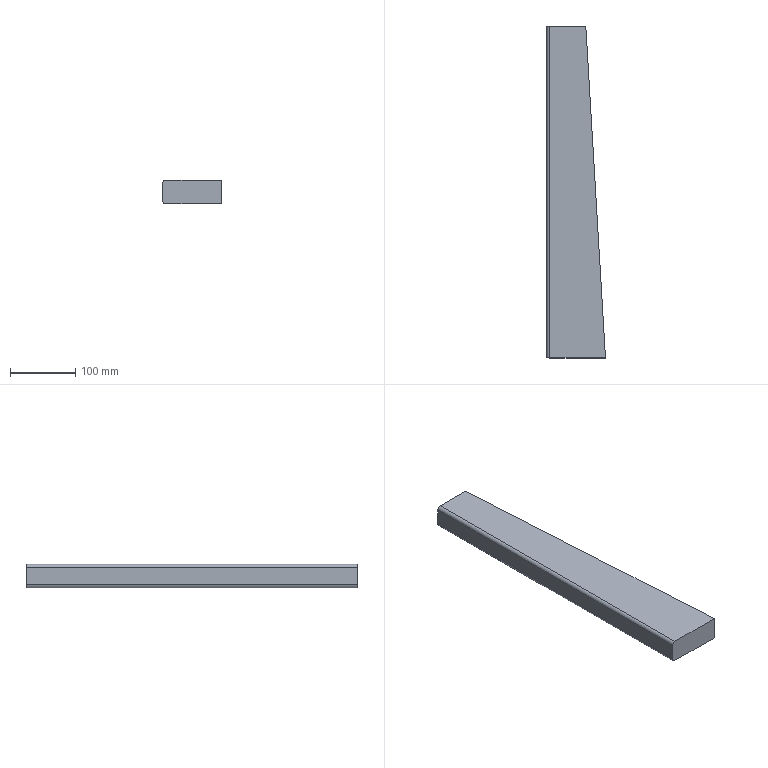Part | STEP file | 07-High-level comb rack 3 | 1 solid | 8 faces | box 90 x 507 x 36 mm | volume 1363460 mm3 | plane 6 | cylinder 2 | commonest cylinder face diameters 10 x2
STEP:
#1=CARTESIAN_POINT('',(0.,0.,0.));
#2=DIRECTION('',(0.,0.,1.));
#3=DIRECTION('',(1.,0.,0.));
#4=AXIS2_PLACEMENT_3D('',#1,#2,#3);
#5=CARTESIAN_POINT('',(0.,0.,31.));
#6=VERTEX_POINT('',#5);
#7=CARTESIAN_POINT('',(0.,0.,5.));
#8=VERTEX_POINT('',#7);
#9=CARTESIAN_POINT('',(0.,0.,36.));
#10=DIRECTION('',(0.,0.,-1.));
#11=VECTOR('',#10,1.);
#12=LINE('',#9,#11);
#13=CARTESIAN_POINT('',(0.,0.,36.));
#14=DIRECTION('',(1.,0.,0.));
#15=DIRECTION('',(0.,1.,0.));
#16=AXIS2_PLACEMENT_3D('',#13,#14,#15);
#17=PLANE('',#16);
#18=CARTESIAN_POINT('',(0.,0.));
#19=DIRECTION('',(0.,-1.));
#20=VECTOR('',#19,1.);
#21=LINE('',#18,#20);
#22=(GEOMETRIC_REPRESENTATION_CONTEXT(2)PARAMETRIC_REPRESENTATION_CONTEXT()REPRESENTATION_CONTEXT('',''));
#23=DEFINITIONAL_REPRESENTATION('',(#21),#22);
#24=PCURVE('',#17,#23);
#25=CARTESIAN_POINT('',(0.,0.,36.));
#26=DIRECTION('',(0.,-1.,0.));
#27=DIRECTION('',(0.,0.,-1.));
#28=AXIS2_PLACEMENT_3D('',#25,#26,#27);
#29=PLANE('',#28);
#30=CARTESIAN_POINT('',(0.,0.));
#31=DIRECTION('',(1.,0.));
#32=VECTOR('',#31,1.);
#33=LINE('',#30,#32);
#34=(GEOMETRIC_REPRESENTATION_CONTEXT(2)PARAMETRIC_REPRESENTATION_CONTEXT()REPRESENTATION_CONTEXT('',''));
#35=DEFINITIONAL_REPRESENTATION('',(#33),#34);
#36=PCURVE('',#29,#35);
#37=SURFACE_CURVE('',#12,(#24,#36),.PCURVE_S1.);
#38=EDGE_CURVE('',#6,#8,#37,.T.);
#39=ORIENTED_EDGE('',*,*,#38,.T.);
#40=CARTESIAN_POINT('',(0.,-507.,5.));
#41=VERTEX_POINT('',#40);
#42=CARTESIAN_POINT('',(0.,0.,5.));
#43=DIRECTION('',(0.,-1.,0.));
#44=VECTOR('',#43,1.);
#45=LINE('',#42,#44);
#46=CARTESIAN_POINT('',(0.,-31.));
#47=DIRECTION('',(-1.,0.));
#48=VECTOR('',#47,1.);
#49=LINE('',#46,#48);
#50=(GEOMETRIC_REPRESENTATION_CONTEXT(2)PARAMETRIC_REPRESENTATION_CONTEXT()REPRESENTATION_CONTEXT('',''));
#51=DEFINITIONAL_REPRESENTATION('',(#49),#50);
#52=PCURVE('',#17,#51);
#53=CARTESIAN_POINT('',(5.,0.,5.));
#54=DIRECTION('',(0.,-1.,0.));
#55=DIRECTION('',(1.,0.,0.));
#56=AXIS2_PLACEMENT_3D('',#53,#54,#55);
#57=CYLINDRICAL_SURFACE('',#56,5.);
#58=CARTESIAN_POINT('',(3.142,0.));
#59=DIRECTION('',(0.,1.));
#60=VECTOR('',#59,1.);
#61=LINE('',#58,#60);
#62=(GEOMETRIC_REPRESENTATION_CONTEXT(2)PARAMETRIC_REPRESENTATION_CONTEXT()REPRESENTATION_CONTEXT('',''));
#63=DEFINITIONAL_REPRESENTATION('',(#61),#62);
#64=PCURVE('',#57,#63);
#65=SURFACE_CURVE('',#45,(#52,#64),.PCURVE_S1.);
#66=EDGE_CURVE('',#8,#41,#65,.T.);
#67=ORIENTED_EDGE('',*,*,#66,.T.);
#68=CARTESIAN_POINT('',(0.,-507.,31.));
#69=VERTEX_POINT('',#68);
#70=CARTESIAN_POINT('',(0.,-507.,36.));
#71=DIRECTION('',(0.,0.,-1.));
#72=VECTOR('',#71,1.);
#73=LINE('',#70,#72);
#74=CARTESIAN_POINT('',(-507.,0.));
#75=DIRECTION('',(0.,-1.));
#76=VECTOR('',#75,1.);
#77=LINE('',#74,#76);
#78=(GEOMETRIC_REPRESENTATION_CONTEXT(2)PARAMETRIC_REPRESENTATION_CONTEXT()REPRESENTATION_CONTEXT('',''));
#79=DEFINITIONAL_REPRESENTATION('',(#77),#78);
#80=PCURVE('',#17,#79);
#81=CARTESIAN_POINT('',(0.,-507.,36.));
#82=DIRECTION('',(0.,1.,0.));
#83=DIRECTION('',(0.,0.,1.));
#84=AXIS2_PLACEMENT_3D('',#81,#82,#83);
#85=PLANE('',#84);
#86=CARTESIAN_POINT('',(0.,0.));
#87=DIRECTION('',(-1.,0.));
#88=VECTOR('',#87,1.);
#89=LINE('',#86,#88);
#90=(GEOMETRIC_REPRESENTATION_CONTEXT(2)PARAMETRIC_REPRESENTATION_CONTEXT()REPRESENTATION_CONTEXT('',''));
#91=DEFINITIONAL_REPRESENTATION('',(#89),#90);
#92=PCURVE('',#85,#91);
#93=SURFACE_CURVE('',#73,(#80,#92),.PCURVE_S1.);
#94=EDGE_CURVE('',#69,#41,#93,.T.);
#95=ORIENTED_EDGE('',*,*,#94,.F.);
#96=CARTESIAN_POINT('',(0.,0.,31.));
#97=DIRECTION('',(0.,1.,0.));
#98=VECTOR('',#97,1.);
#99=LINE('',#96,#98);
#100=CARTESIAN_POINT('',(0.,-5.));
#101=DIRECTION('',(1.,0.));
#102=VECTOR('',#101,1.);
#103=LINE('',#100,#102);
#104=(GEOMETRIC_REPRESENTATION_CONTEXT(2)PARAMETRIC_REPRESENTATION_CONTEXT()REPRESENTATION_CONTEXT('',''));
#105=DEFINITIONAL_REPRESENTATION('',(#103),#104);
#106=PCURVE('',#17,#105);
#107=CARTESIAN_POINT('',(5.,0.,31.));
#108=DIRECTION('',(0.,1.,0.));
#109=DIRECTION('',(-1.,0.,0.));
#110=AXIS2_PLACEMENT_3D('',#107,#108,#109);
#111=CYLINDRICAL_SURFACE('',#110,5.);
#112=CARTESIAN_POINT('',(0.,0.));
#113=DIRECTION('',(0.,1.));
#114=VECTOR('',#113,1.);
#115=LINE('',#112,#114);
#116=(GEOMETRIC_REPRESENTATION_CONTEXT(2)PARAMETRIC_REPRESENTATION_CONTEXT()REPRESENTATION_CONTEXT('',''));
#117=DEFINITIONAL_REPRESENTATION('',(#115),#116);
#118=PCURVE('',#111,#117);
#119=SURFACE_CURVE('',#99,(#106,#118),.PCURVE_S1.);
#120=EDGE_CURVE('',#69,#6,#119,.T.);
#121=ORIENTED_EDGE('',*,*,#120,.T.);
#122=EDGE_LOOP('',(#39,#67,#95,#121));
#123=FACE_BOUND('',#122,.T.);
#124=ADVANCED_FACE('',(#123),#17,.F.);
#125=ORIENTED_EDGE('',*,*,#94,.T.);
#126=CARTESIAN_POINT('',(5.,-507.,0.));
#127=VERTEX_POINT('',#126);
#128=CARTESIAN_POINT('',(5.,-507.,5.));
#129=DIRECTION('',(0.,-1.,0.));
#130=DIRECTION('',(0.,0.,1.));
#131=AXIS2_PLACEMENT_3D('',#128,#129,#130);
#132=CIRCLE('',#131,5.);
#133=CARTESIAN_POINT('',(-26.,5.));
#134=CARTESIAN_POINT('',(-26.,-3.66));
#135=CARTESIAN_POINT('',(-33.5,0.6699));
#136=CARTESIAN_POINT('',(-41.,5.));
#137=CARTESIAN_POINT('',(-33.5,9.33));
#138=CARTESIAN_POINT('',(-26.,13.66));
#139=CARTESIAN_POINT('',(-26.,5.));
#140=(BOUNDED_CURVE()B_SPLINE_CURVE(2,(#133,#134,#135,#136,#137,#138,#139),.UNSPECIFIED.,.T.,.F.)B_SPLINE_CURVE_WITH_KNOTS((1,2,2,2,2,1),(-2.094,0.,2.094,4.189,6.283,8.378),.UNSPECIFIED.)CURVE()GEOMETRIC_REPRESENTATION_ITEM()RATIONAL_B_SPLINE_CURVE((1.,0.5,1.,0.5,1.,0.5,1.))REPRESENTATION_ITEM(''));
#141=(GEOMETRIC_REPRESENTATION_CONTEXT(2)PARAMETRIC_REPRESENTATION_CONTEXT()REPRESENTATION_CONTEXT('',''));
#142=DEFINITIONAL_REPRESENTATION('',(#140),#141);
#143=PCURVE('',#85,#142);
#144=CARTESIAN_POINT('',(1.571,507.));
#145=DIRECTION('',(1.,0.));
#146=VECTOR('',#145,1.);
#147=LINE('',#144,#146);
#148=(GEOMETRIC_REPRESENTATION_CONTEXT(2)PARAMETRIC_REPRESENTATION_CONTEXT()REPRESENTATION_CONTEXT('',''));
#149=DEFINITIONAL_REPRESENTATION('',(#147),#148);
#150=PCURVE('',#57,#149);
#151=SURFACE_CURVE('',#132,(#143,#150),.PCURVE_S1.);
#152=EDGE_CURVE('',#41,#127,#151,.T.);
#153=ORIENTED_EDGE('',*,*,#152,.T.);
#154=CARTESIAN_POINT('',(90.,-507.,0.));
#155=VERTEX_POINT('',#154);
#156=CARTESIAN_POINT('',(0.,-507.,0.));
#157=DIRECTION('',(1.,0.,0.));
#158=VECTOR('',#157,1.);
#159=LINE('',#156,#158);
#160=CARTESIAN_POINT('',(-36.,0.));
#161=DIRECTION('',(0.,1.));
#162=VECTOR('',#161,1.);
#163=LINE('',#160,#162);
#164=(GEOMETRIC_REPRESENTATION_CONTEXT(2)PARAMETRIC_REPRESENTATION_CONTEXT()REPRESENTATION_CONTEXT('',''));
#165=DEFINITIONAL_REPRESENTATION('',(#163),#164);
#166=PCURVE('',#85,#165);
#167=CARTESIAN_POINT('',(0.,0.,0.));
#168=DIRECTION('',(0.,0.,1.));
#169=DIRECTION('',(1.,0.,0.));
#170=AXIS2_PLACEMENT_3D('',#167,#168,#169);
#171=PLANE('',#170);
#172=CARTESIAN_POINT('',(0.,-507.));
#173=DIRECTION('',(1.,0.));
#174=VECTOR('',#173,1.);
#175=LINE('',#172,#174);
#176=(GEOMETRIC_REPRESENTATION_CONTEXT(2)PARAMETRIC_REPRESENTATION_CONTEXT()REPRESENTATION_CONTEXT('',''));
#177=DEFINITIONAL_REPRESENTATION('',(#175),#176);
#178=PCURVE('',#171,#177);
#179=SURFACE_CURVE('',#159,(#166,#178),.PCURVE_S1.);
#180=EDGE_CURVE('',#127,#155,#179,.T.);
#181=ORIENTED_EDGE('',*,*,#180,.T.);
#182=CARTESIAN_POINT('',(90.,-507.,36.));
#183=VERTEX_POINT('',#182);
#184=CARTESIAN_POINT('',(90.,-507.,36.));
#185=DIRECTION('',(0.,0.,-1.));
#186=VECTOR('',#185,1.);
#187=LINE('',#184,#186);
#188=CARTESIAN_POINT('',(0.,90.));
#189=DIRECTION('',(-1.,0.));
#190=VECTOR('',#189,1.);
#191=LINE('',#188,#190);
#192=(GEOMETRIC_REPRESENTATION_CONTEXT(2)PARAMETRIC_REPRESENTATION_CONTEXT()REPRESENTATION_CONTEXT('',''));
#193=DEFINITIONAL_REPRESENTATION('',(#191),#192);
#194=PCURVE('',#85,#193);
#195=CARTESIAN_POINT('',(60.,0.,36.));
#196=DIRECTION('',(-0.9983,-0.05907,0.));
#197=DIRECTION('',(0.05907,-0.9983,0.));
#198=AXIS2_PLACEMENT_3D('',#195,#196,#197);
#199=PLANE('',#198);
#200=CARTESIAN_POINT('',(507.887,0.));
#201=DIRECTION('',(0.,-1.));
#202=VECTOR('',#201,1.);
#203=LINE('',#200,#202);
#204=(GEOMETRIC_REPRESENTATION_CONTEXT(2)PARAMETRIC_REPRESENTATION_CONTEXT()REPRESENTATION_CONTEXT('',''));
#205=DEFINITIONAL_REPRESENTATION('',(#203),#204);
#206=PCURVE('',#199,#205);
#207=SURFACE_CURVE('',#187,(#194,#206),.PCURVE_S1.);
#208=EDGE_CURVE('',#183,#155,#207,.T.);
#209=ORIENTED_EDGE('',*,*,#208,.F.);
#210=CARTESIAN_POINT('',(5.,-507.,36.));
#211=VERTEX_POINT('',#210);
#212=CARTESIAN_POINT('',(0.,-507.,36.));
#213=DIRECTION('',(1.,0.,0.));
#214=VECTOR('',#213,1.);
#215=LINE('',#212,#214);
#216=CARTESIAN_POINT('',(0.,0.));
#217=DIRECTION('',(0.,1.));
#218=VECTOR('',#217,1.);
#219=LINE('',#216,#218);
#220=(GEOMETRIC_REPRESENTATION_CONTEXT(2)PARAMETRIC_REPRESENTATION_CONTEXT()REPRESENTATION_CONTEXT('',''));
#221=DEFINITIONAL_REPRESENTATION('',(#219),#220);
#222=PCURVE('',#85,#221);
#223=CARTESIAN_POINT('',(0.,0.,36.));
#224=DIRECTION('',(0.,0.,1.));
#225=DIRECTION('',(1.,0.,0.));
#226=AXIS2_PLACEMENT_3D('',#223,#224,#225);
#227=PLANE('',#226);
#228=CARTESIAN_POINT('',(0.,-507.));
#229=DIRECTION('',(1.,0.));
#230=VECTOR('',#229,1.);
#231=LINE('',#228,#230);
#232=(GEOMETRIC_REPRESENTATION_CONTEXT(2)PARAMETRIC_REPRESENTATION_CONTEXT()REPRESENTATION_CONTEXT('',''));
#233=DEFINITIONAL_REPRESENTATION('',(#231),#232);
#234=PCURVE('',#227,#233);
#235=SURFACE_CURVE('',#215,(#222,#234),.PCURVE_S1.);
#236=EDGE_CURVE('',#211,#183,#235,.T.);
#237=ORIENTED_EDGE('',*,*,#236,.F.);
#238=CARTESIAN_POINT('',(5.,-507.,31.));
#239=DIRECTION('',(0.,-1.,0.));
#240=DIRECTION('',(0.,0.,1.));
#241=AXIS2_PLACEMENT_3D('',#238,#239,#240);
#242=CIRCLE('',#241,5.);
#243=CARTESIAN_POINT('',(0.,5.));
#244=CARTESIAN_POINT('',(0.,-3.66));
#245=CARTESIAN_POINT('',(-7.5,0.6699));
#246=CARTESIAN_POINT('',(-15.,5.));
#247=CARTESIAN_POINT('',(-7.5,9.33));
#248=CARTESIAN_POINT('',(0.,13.66));
#249=CARTESIAN_POINT('',(0.,5.));
#250=(BOUNDED_CURVE()B_SPLINE_CURVE(2,(#243,#244,#245,#246,#247,#248,#249),.UNSPECIFIED.,.T.,.F.)B_SPLINE_CURVE_WITH_KNOTS((1,2,2,2,2,1),(-2.094,0.,2.094,4.189,6.283,8.378),.UNSPECIFIED.)CURVE()GEOMETRIC_REPRESENTATION_ITEM()RATIONAL_B_SPLINE_CURVE((1.,0.5,1.,0.5,1.,0.5,1.))REPRESENTATION_ITEM(''));
#251=(GEOMETRIC_REPRESENTATION_CONTEXT(2)PARAMETRIC_REPRESENTATION_CONTEXT()REPRESENTATION_CONTEXT('',''));
#252=DEFINITIONAL_REPRESENTATION('',(#250),#251);
#253=PCURVE('',#85,#252);
#254=CARTESIAN_POINT('',(1.571,-507.));
#255=DIRECTION('',(-1.,0.));
#256=VECTOR('',#255,1.);
#257=LINE('',#254,#256);
#258=(GEOMETRIC_REPRESENTATION_CONTEXT(2)PARAMETRIC_REPRESENTATION_CONTEXT()REPRESENTATION_CONTEXT('',''));
#259=DEFINITIONAL_REPRESENTATION('',(#257),#258);
#260=PCURVE('',#111,#259);
#261=SURFACE_CURVE('',#242,(#253,#260),.PCURVE_S1.);
#262=EDGE_CURVE('',#211,#69,#261,.T.);
#263=ORIENTED_EDGE('',*,*,#262,.T.);
#264=EDGE_LOOP('',(#125,#153,#181,#209,#237,#263));
#265=FACE_BOUND('',#264,.T.);
#266=ADVANCED_FACE('',(#265),#85,.F.);
#267=CARTESIAN_POINT('',(60.,0.,0.));
#268=VERTEX_POINT('',#267);
#269=CARTESIAN_POINT('',(60.,0.,0.));
#270=DIRECTION('',(-0.05907,0.9983,0.));
#271=VECTOR('',#270,1.);
#272=LINE('',#269,#271);
#273=CARTESIAN_POINT('',(0.,-36.));
#274=DIRECTION('',(-1.,0.));
#275=VECTOR('',#274,1.);
#276=LINE('',#273,#275);
#277=(GEOMETRIC_REPRESENTATION_CONTEXT(2)PARAMETRIC_REPRESENTATION_CONTEXT()REPRESENTATION_CONTEXT('',''));
#278=DEFINITIONAL_REPRESENTATION('',(#276),#277);
#279=PCURVE('',#199,#278);
#280=CARTESIAN_POINT('',(60.,0.));
#281=DIRECTION('',(-0.05907,0.9983));
#282=VECTOR('',#281,1.);
#283=LINE('',#280,#282);
#284=(GEOMETRIC_REPRESENTATION_CONTEXT(2)PARAMETRIC_REPRESENTATION_CONTEXT()REPRESENTATION_CONTEXT('',''));
#285=DEFINITIONAL_REPRESENTATION('',(#283),#284);
#286=PCURVE('',#171,#285);
#287=SURFACE_CURVE('',#272,(#279,#286),.PCURVE_S1.);
#288=EDGE_CURVE('',#155,#268,#287,.T.);
#289=ORIENTED_EDGE('',*,*,#288,.T.);
#290=CARTESIAN_POINT('',(60.,0.,36.));
#291=VERTEX_POINT('',#290);
#292=CARTESIAN_POINT('',(60.,0.,36.));
#293=DIRECTION('',(0.,0.,-1.));
#294=VECTOR('',#293,1.);
#295=LINE('',#292,#294);
#296=CARTESIAN_POINT('',(0.,0.));
#297=DIRECTION('',(0.,-1.));
#298=VECTOR('',#297,1.);
#299=LINE('',#296,#298);
#300=(GEOMETRIC_REPRESENTATION_CONTEXT(2)PARAMETRIC_REPRESENTATION_CONTEXT()REPRESENTATION_CONTEXT('',''));
#301=DEFINITIONAL_REPRESENTATION('',(#299),#300);
#302=PCURVE('',#199,#301);
#303=CARTESIAN_POINT('',(0.,60.));
#304=DIRECTION('',(1.,0.));
#305=VECTOR('',#304,1.);
#306=LINE('',#303,#305);
#307=(GEOMETRIC_REPRESENTATION_CONTEXT(2)PARAMETRIC_REPRESENTATION_CONTEXT()REPRESENTATION_CONTEXT('',''));
#308=DEFINITIONAL_REPRESENTATION('',(#306),#307);
#309=PCURVE('',#29,#308);
#310=SURFACE_CURVE('',#295,(#302,#309),.PCURVE_S1.);
#311=EDGE_CURVE('',#291,#268,#310,.T.);
#312=ORIENTED_EDGE('',*,*,#311,.F.);
#313=CARTESIAN_POINT('',(60.,0.,36.));
#314=DIRECTION('',(-0.05907,0.9983,0.));
#315=VECTOR('',#314,1.);
#316=LINE('',#313,#315);
#317=CARTESIAN_POINT('',(0.,0.));
#318=DIRECTION('',(-1.,0.));
#319=VECTOR('',#318,1.);
#320=LINE('',#317,#319);
#321=(GEOMETRIC_REPRESENTATION_CONTEXT(2)PARAMETRIC_REPRESENTATION_CONTEXT()REPRESENTATION_CONTEXT('',''));
#322=DEFINITIONAL_REPRESENTATION('',(#320),#321);
#323=PCURVE('',#199,#322);
#324=CARTESIAN_POINT('',(60.,0.));
#325=DIRECTION('',(-0.05907,0.9983));
#326=VECTOR('',#325,1.);
#327=LINE('',#324,#326);
#328=(GEOMETRIC_REPRESENTATION_CONTEXT(2)PARAMETRIC_REPRESENTATION_CONTEXT()REPRESENTATION_CONTEXT('',''));
#329=DEFINITIONAL_REPRESENTATION('',(#327),#328);
#330=PCURVE('',#227,#329);
#331=SURFACE_CURVE('',#316,(#323,#330),.PCURVE_S1.);
#332=EDGE_CURVE('',#183,#291,#331,.T.);
#333=ORIENTED_EDGE('',*,*,#332,.F.);
#334=ORIENTED_EDGE('',*,*,#208,.T.);
#335=EDGE_LOOP('',(#289,#312,#333,#334));
#336=FACE_BOUND('',#335,.T.);
#337=ADVANCED_FACE('',(#336),#199,.F.);
#338=CARTESIAN_POINT('',(5.,0.,0.));
#339=VERTEX_POINT('',#338);
#340=CARTESIAN_POINT('',(0.,0.,0.));
#341=DIRECTION('',(-1.,0.,0.));
#342=VECTOR('',#341,1.);
#343=LINE('',#340,#342);
#344=CARTESIAN_POINT('',(36.,0.));
#345=DIRECTION('',(0.,-1.));
#346=VECTOR('',#345,1.);
#347=LINE('',#344,#346);
#348=(GEOMETRIC_REPRESENTATION_CONTEXT(2)PARAMETRIC_REPRESENTATION_CONTEXT()REPRESENTATION_CONTEXT('',''));
#349=DEFINITIONAL_REPRESENTATION('',(#347),#348);
#350=PCURVE('',#29,#349);
#351=CARTESIAN_POINT('',(0.,0.));
#352=DIRECTION('',(-1.,0.));
#353=VECTOR('',#352,1.);
#354=LINE('',#351,#353);
#355=(GEOMETRIC_REPRESENTATION_CONTEXT(2)PARAMETRIC_REPRESENTATION_CONTEXT()REPRESENTATION_CONTEXT('',''));
#356=DEFINITIONAL_REPRESENTATION('',(#354),#355);
#357=PCURVE('',#171,#356);
#358=SURFACE_CURVE('',#343,(#350,#357),.PCURVE_S1.);
#359=EDGE_CURVE('',#268,#339,#358,.T.);
#360=ORIENTED_EDGE('',*,*,#359,.T.);
#361=CARTESIAN_POINT('',(5.,0.,5.));
#362=DIRECTION('',(0.,1.,0.));
#363=DIRECTION('',(0.,0.,-1.));
#364=AXIS2_PLACEMENT_3D('',#361,#362,#363);
#365=CIRCLE('',#364,5.);
#366=CARTESIAN_POINT('',(36.,5.));
#367=CARTESIAN_POINT('',(36.,-3.66));
#368=CARTESIAN_POINT('',(28.5,0.6699));
#369=CARTESIAN_POINT('',(21.,5.));
#370=CARTESIAN_POINT('',(28.5,9.33));
#371=CARTESIAN_POINT('',(36.,13.66));
#372=CARTESIAN_POINT('',(36.,5.));
#373=(BOUNDED_CURVE()B_SPLINE_CURVE(2,(#366,#367,#368,#369,#370,#371,#372),.UNSPECIFIED.,.T.,.F.)B_SPLINE_CURVE_WITH_KNOTS((1,2,2,2,2,1),(-2.094,0.,2.094,4.189,6.283,8.378),.UNSPECIFIED.)CURVE()GEOMETRIC_REPRESENTATION_ITEM()RATIONAL_B_SPLINE_CURVE((1.,0.5,1.,0.5,1.,0.5,1.))REPRESENTATION_ITEM(''));
#374=(GEOMETRIC_REPRESENTATION_CONTEXT(2)PARAMETRIC_REPRESENTATION_CONTEXT()REPRESENTATION_CONTEXT('',''));
#375=DEFINITIONAL_REPRESENTATION('',(#373),#374);
#376=PCURVE('',#29,#375);
#377=CARTESIAN_POINT('',(4.712,0.));
#378=DIRECTION('',(-1.,0.));
#379=VECTOR('',#378,1.);
#380=LINE('',#377,#379);
#381=(GEOMETRIC_REPRESENTATION_CONTEXT(2)PARAMETRIC_REPRESENTATION_CONTEXT()REPRESENTATION_CONTEXT('',''));
#382=DEFINITIONAL_REPRESENTATION('',(#380),#381);
#383=PCURVE('',#57,#382);
#384=SURFACE_CURVE('',#365,(#376,#383),.PCURVE_S1.);
#385=EDGE_CURVE('',#339,#8,#384,.T.);
#386=ORIENTED_EDGE('',*,*,#385,.T.);
#387=ORIENTED_EDGE('',*,*,#38,.F.);
#388=CARTESIAN_POINT('',(5.,0.,36.));
#389=VERTEX_POINT('',#388);
#390=CARTESIAN_POINT('',(5.,0.,31.));
#391=DIRECTION('',(0.,1.,0.));
#392=DIRECTION('',(0.,0.,-1.));
#393=AXIS2_PLACEMENT_3D('',#390,#391,#392);
#394=CIRCLE('',#393,5.);
#395=CARTESIAN_POINT('',(10.,5.));
#396=CARTESIAN_POINT('',(10.,-3.66));
#397=CARTESIAN_POINT('',(2.5,0.6699));
#398=CARTESIAN_POINT('',(-5.,5.));
#399=CARTESIAN_POINT('',(2.5,9.33));
#400=CARTESIAN_POINT('',(10.,13.66));
#401=CARTESIAN_POINT('',(10.,5.));
#402=(BOUNDED_CURVE()B_SPLINE_CURVE(2,(#395,#396,#397,#398,#399,#400,#401),.UNSPECIFIED.,.T.,.F.)B_SPLINE_CURVE_WITH_KNOTS((1,2,2,2,2,1),(-2.094,0.,2.094,4.189,6.283,8.378),.UNSPECIFIED.)CURVE()GEOMETRIC_REPRESENTATION_ITEM()RATIONAL_B_SPLINE_CURVE((1.,0.5,1.,0.5,1.,0.5,1.))REPRESENTATION_ITEM(''));
#403=(GEOMETRIC_REPRESENTATION_CONTEXT(2)PARAMETRIC_REPRESENTATION_CONTEXT()REPRESENTATION_CONTEXT('',''));
#404=DEFINITIONAL_REPRESENTATION('',(#402),#403);
#405=PCURVE('',#29,#404);
#406=CARTESIAN_POINT('',(-1.571,0.));
#407=DIRECTION('',(1.,0.));
#408=VECTOR('',#407,1.);
#409=LINE('',#406,#408);
#410=(GEOMETRIC_REPRESENTATION_CONTEXT(2)PARAMETRIC_REPRESENTATION_CONTEXT()REPRESENTATION_CONTEXT('',''));
#411=DEFINITIONAL_REPRESENTATION('',(#409),#410);
#412=PCURVE('',#111,#411);
#413=SURFACE_CURVE('',#394,(#405,#412),.PCURVE_S1.);
#414=EDGE_CURVE('',#6,#389,#413,.T.);
#415=ORIENTED_EDGE('',*,*,#414,.T.);
#416=CARTESIAN_POINT('',(0.,0.,36.));
#417=DIRECTION('',(-1.,0.,0.));
#418=VECTOR('',#417,1.);
#419=LINE('',#416,#418);
#420=CARTESIAN_POINT('',(0.,0.));
#421=DIRECTION('',(0.,-1.));
#422=VECTOR('',#421,1.);
#423=LINE('',#420,#422);
#424=(GEOMETRIC_REPRESENTATION_CONTEXT(2)PARAMETRIC_REPRESENTATION_CONTEXT()REPRESENTATION_CONTEXT('',''));
#425=DEFINITIONAL_REPRESENTATION('',(#423),#424);
#426=PCURVE('',#29,#425);
#427=CARTESIAN_POINT('',(0.,0.));
#428=DIRECTION('',(-1.,0.));
#429=VECTOR('',#428,1.);
#430=LINE('',#427,#429);
#431=(GEOMETRIC_REPRESENTATION_CONTEXT(2)PARAMETRIC_REPRESENTATION_CONTEXT()REPRESENTATION_CONTEXT('',''));
#432=DEFINITIONAL_REPRESENTATION('',(#430),#431);
#433=PCURVE('',#227,#432);
#434=SURFACE_CURVE('',#419,(#426,#433),.PCURVE_S1.);
#435=EDGE_CURVE('',#291,#389,#434,.T.);
#436=ORIENTED_EDGE('',*,*,#435,.F.);
#437=ORIENTED_EDGE('',*,*,#311,.T.);
#438=EDGE_LOOP('',(#360,#386,#387,#415,#436,#437));
#439=FACE_BOUND('',#438,.T.);
#440=ADVANCED_FACE('',(#439),#29,.F.);
#441=ORIENTED_EDGE('',*,*,#435,.T.);
#442=CARTESIAN_POINT('',(5.,-507.,36.));
#443=DIRECTION('',(0.,-1.,0.));
#444=VECTOR('',#443,1.);
#445=LINE('',#442,#444);
#446=CARTESIAN_POINT('',(5.,-507.));
#447=DIRECTION('',(0.,-1.));
#448=VECTOR('',#447,1.);
#449=LINE('',#446,#448);
#450=(GEOMETRIC_REPRESENTATION_CONTEXT(2)PARAMETRIC_REPRESENTATION_CONTEXT()REPRESENTATION_CONTEXT('',''));
#451=DEFINITIONAL_REPRESENTATION('',(#449),#450);
#452=PCURVE('',#227,#451);
#453=CARTESIAN_POINT('',(1.571,-507.));
#454=DIRECTION('',(0.,-1.));
#455=VECTOR('',#454,1.);
#456=LINE('',#453,#455);
#457=(GEOMETRIC_REPRESENTATION_CONTEXT(2)PARAMETRIC_REPRESENTATION_CONTEXT()REPRESENTATION_CONTEXT('',''));
#458=DEFINITIONAL_REPRESENTATION('',(#456),#457);
#459=PCURVE('',#111,#458);
#460=SURFACE_CURVE('',#445,(#452,#459),.PCURVE_S1.);
#461=EDGE_CURVE('',#389,#211,#460,.T.);
#462=ORIENTED_EDGE('',*,*,#461,.T.);
#463=ORIENTED_EDGE('',*,*,#236,.T.);
#464=ORIENTED_EDGE('',*,*,#332,.T.);
#465=EDGE_LOOP('',(#441,#462,#463,#464));
#466=FACE_BOUND('',#465,.T.);
#467=ADVANCED_FACE('',(#466),#227,.T.);
#468=ORIENTED_EDGE('',*,*,#180,.F.);
#469=CARTESIAN_POINT('',(5.,0.,0.));
#470=DIRECTION('',(0.,1.,0.));
#471=VECTOR('',#470,1.);
#472=LINE('',#469,#471);
#473=CARTESIAN_POINT('',(5.,0.));
#474=DIRECTION('',(0.,1.));
#475=VECTOR('',#474,1.);
#476=LINE('',#473,#475);
#477=(GEOMETRIC_REPRESENTATION_CONTEXT(2)PARAMETRIC_REPRESENTATION_CONTEXT()REPRESENTATION_CONTEXT('',''));
#478=DEFINITIONAL_REPRESENTATION('',(#476),#477);
#479=PCURVE('',#171,#478);
#480=CARTESIAN_POINT('',(4.712,0.));
#481=DIRECTION('',(0.,-1.));
#482=VECTOR('',#481,1.);
#483=LINE('',#480,#482);
#484=(GEOMETRIC_REPRESENTATION_CONTEXT(2)PARAMETRIC_REPRESENTATION_CONTEXT()REPRESENTATION_CONTEXT('',''));
#485=DEFINITIONAL_REPRESENTATION('',(#483),#484);
#486=PCURVE('',#57,#485);
#487=SURFACE_CURVE('',#472,(#479,#486),.PCURVE_S1.);
#488=EDGE_CURVE('',#127,#339,#487,.T.);
#489=ORIENTED_EDGE('',*,*,#488,.T.);
#490=ORIENTED_EDGE('',*,*,#359,.F.);
#491=ORIENTED_EDGE('',*,*,#288,.F.);
#492=EDGE_LOOP('',(#468,#489,#490,#491));
#493=FACE_BOUND('',#492,.T.);
#494=ADVANCED_FACE('',(#493),#171,.F.);
#495=ORIENTED_EDGE('',*,*,#385,.F.);
#496=ORIENTED_EDGE('',*,*,#488,.F.);
#497=ORIENTED_EDGE('',*,*,#152,.F.);
#498=ORIENTED_EDGE('',*,*,#66,.F.);
#499=EDGE_LOOP('',(#495,#496,#497,#498));
#500=FACE_BOUND('',#499,.T.);
#501=ADVANCED_FACE('',(#500),#57,.T.);
#502=ORIENTED_EDGE('',*,*,#414,.F.);
#503=ORIENTED_EDGE('',*,*,#120,.F.);
#504=ORIENTED_EDGE('',*,*,#262,.F.);
#505=ORIENTED_EDGE('',*,*,#461,.F.);
#506=EDGE_LOOP('',(#502,#503,#504,#505));
#507=FACE_BOUND('',#506,.T.);
#508=ADVANCED_FACE('',(#507),#111,.T.);
#509=CLOSED_SHELL('',(#124,#266,#337,#440,#467,#494,#501,#508));
#510=MANIFOLD_SOLID_BREP('',#509);
#511=(LENGTH_UNIT()NAMED_UNIT(*)SI_UNIT(.MILLI.,.METRE.));
#512=UNCERTAINTY_MEASURE_WITH_UNIT(LENGTH_MEASURE(0.0000001),#511,'','');
#513=(NAMED_UNIT(*)PLANE_ANGLE_UNIT()SI_UNIT($,.RADIAN.));
#514=(NAMED_UNIT(*)SI_UNIT($,.STERADIAN.)SOLID_ANGLE_UNIT());
#515=(GEOMETRIC_REPRESENTATION_CONTEXT(3)GLOBAL_UNCERTAINTY_ASSIGNED_CONTEXT((#512))GLOBAL_UNIT_ASSIGNED_CONTEXT((#511,#513,#514))REPRESENTATION_CONTEXT('',''));
#516=ADVANCED_BREP_SHAPE_REPRESENTATION('',(#4,#510),#515);